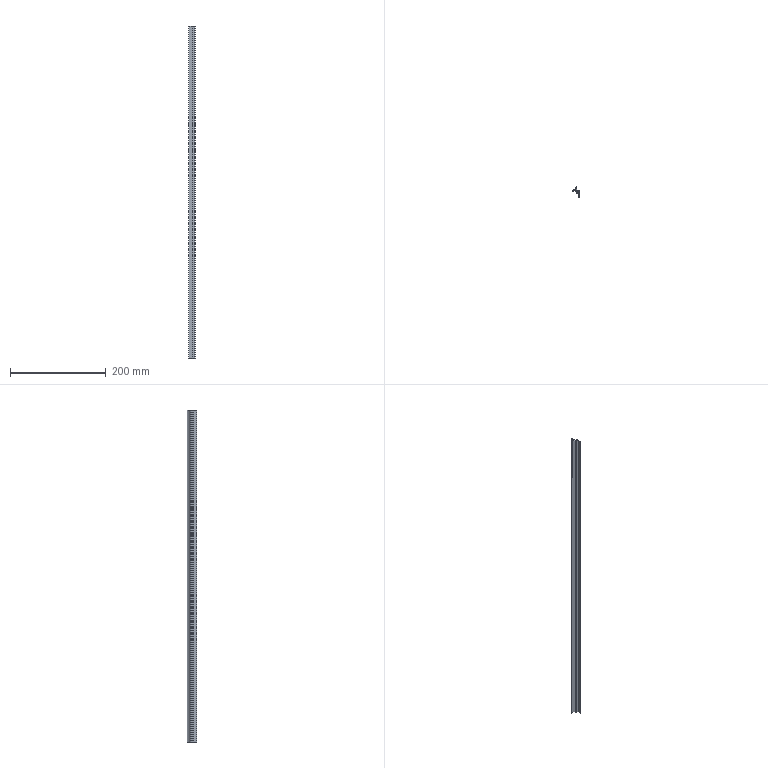Part | SolidWorks | features BaseBody 1, ICE 1, MoveFace 1 | 1 solid | 27 faces | box 14 x 20.3 x 692 mm | volume 35234 mm3 | plane 20 | cylinder 7 | commonest cylinder face diameters 0.387 x2 0.8 x2 0.4 x1 20 x1 22 x1
STEP:
#1=CARTESIAN_POINT('',(-5.304,-0.625,200.));
#2=VERTEX_POINT('',#1);
#3=CARTESIAN_POINT('',(-5.449,-0.8125,200.));
#4=VERTEX_POINT('',#3);
#5=CARTESIAN_POINT('',(-5.255,-0.8125,200.));
#6=DIRECTION('',(0.,0.,1.));
#7=DIRECTION('',(-1.,0.,0.));
#8=AXIS2_PLACEMENT_3D('',#5,#6,#7);
#9=CIRCLE('',#8,0.1937);
#10=EDGE_CURVE('',#2,#4,#9,.T.);
#11=ORIENTED_EDGE('',*,*,#10,.T.);
#12=CARTESIAN_POINT('',(-5.449,-0.8125,-492.));
#13=VERTEX_POINT('',#12);
#14=CARTESIAN_POINT('',(-5.449,-0.8125,230.));
#15=DIRECTION('',(0.,0.,-1.));
#16=VECTOR('',#15,1000.);
#17=LINE('',#14,#16);
#18=EDGE_CURVE('',#4,#13,#17,.T.);
#19=ORIENTED_EDGE('',*,*,#18,.T.);
#20=CARTESIAN_POINT('',(-5.304,-0.625,-492.));
#21=VERTEX_POINT('',#20);
#22=CARTESIAN_POINT('',(-5.255,-0.8125,-492.));
#23=DIRECTION('',(0.,0.,-1.));
#24=DIRECTION('',(1.,0.,0.));
#25=AXIS2_PLACEMENT_3D('',#22,#23,#24);
#26=CIRCLE('',#25,0.1937);
#27=EDGE_CURVE('',#13,#21,#26,.T.);
#28=ORIENTED_EDGE('',*,*,#27,.T.);
#29=CARTESIAN_POINT('',(-5.304,-0.625,230.));
#30=DIRECTION('',(0.,0.,-1.));
#31=VECTOR('',#30,1000.);
#32=LINE('',#29,#31);
#33=EDGE_CURVE('',#2,#21,#32,.T.);
#34=ORIENTED_EDGE('',*,*,#33,.F.);
#35=EDGE_LOOP('',(#11,#19,#28,#34));
#36=FACE_OUTER_BOUND('',#35,.T.);
#37=CARTESIAN_POINT('',(-5.255,-0.8125,230.));
#38=DIRECTION('',(0.,0.,-1.));
#39=DIRECTION('',(-1.,0.,0.));
#40=AXIS2_PLACEMENT_3D('',#37,#38,#39);
#41=CYLINDRICAL_SURFACE('',#40,0.1937);
#42=ADVANCED_FACE('',(#36),#41,.F.);
#43=CARTESIAN_POINT('',(5.,-1.,-492.));
#44=VERTEX_POINT('',#43);
#45=CARTESIAN_POINT('',(5.,-14.3,-492.));
#46=VERTEX_POINT('',#45);
#47=CARTESIAN_POINT('',(5.,29.623,-492.));
#48=DIRECTION('',(0.,-1.,0.));
#49=VECTOR('',#48,1000.);
#50=LINE('',#47,#49);
#51=EDGE_CURVE('',#44,#46,#50,.T.);
#52=ORIENTED_EDGE('',*,*,#51,.F.);
#53=CARTESIAN_POINT('',(5.,-1.,200.));
#54=VERTEX_POINT('',#53);
#55=CARTESIAN_POINT('',(5.,-1.,230.));
#56=DIRECTION('',(0.,0.,-1.));
#57=VECTOR('',#56,1000.);
#58=LINE('',#55,#57);
#59=EDGE_CURVE('',#54,#44,#58,.T.);
#60=ORIENTED_EDGE('',*,*,#59,.F.);
#61=CARTESIAN_POINT('',(5.,-14.3,200.));
#62=VERTEX_POINT('',#61);
#63=CARTESIAN_POINT('',(5.,-14.3,200.));
#64=DIRECTION('',(0.,1.,0.));
#65=VECTOR('',#64,1000.);
#66=LINE('',#63,#65);
#67=EDGE_CURVE('',#62,#54,#66,.T.);
#68=ORIENTED_EDGE('',*,*,#67,.F.);
#69=CARTESIAN_POINT('',(5.,-14.3,230.));
#70=DIRECTION('',(0.,0.,1.));
#71=VECTOR('',#70,1000.);
#72=LINE('',#69,#71);
#73=EDGE_CURVE('',#46,#62,#72,.T.);
#74=ORIENTED_EDGE('',*,*,#73,.F.);
#75=EDGE_LOOP('',(#52,#60,#68,#74));
#76=FACE_OUTER_BOUND('',#75,.T.);
#77=CARTESIAN_POINT('',(5.,-14.3,230.));
#78=DIRECTION('',(-1.,0.,0.));
#79=DIRECTION('',(0.,0.,1.));
#80=AXIS2_PLACEMENT_3D('',#77,#78,#79);
#81=PLANE('',#80);
#82=ADVANCED_FACE('',(#76),#81,.F.);
#83=CARTESIAN_POINT('',(-9.,-2.,-492.));
#84=VERTEX_POINT('',#83);
#85=CARTESIAN_POINT('',(-9.,-2.,200.));
#86=VERTEX_POINT('',#85);
#87=CARTESIAN_POINT('',(-9.,-2.,230.));
#88=DIRECTION('',(0.,0.,1.));
#89=VECTOR('',#88,1000.);
#90=LINE('',#87,#89);
#91=EDGE_CURVE('',#84,#86,#90,.T.);
#92=ORIENTED_EDGE('',*,*,#91,.F.);
#93=CARTESIAN_POINT('',(0.9,-2.,-492.));
#94=VERTEX_POINT('',#93);
#95=CARTESIAN_POINT('',(5.,-2.,-492.));
#96=DIRECTION('',(-1.,0.,0.));
#97=VECTOR('',#96,1000.);
#98=LINE('',#95,#97);
#99=EDGE_CURVE('',#94,#84,#98,.T.);
#100=ORIENTED_EDGE('',*,*,#99,.F.);
#101=CARTESIAN_POINT('',(0.9,-2.,200.));
#102=VERTEX_POINT('',#101);
#103=CARTESIAN_POINT('',(0.9,-2.,230.));
#104=DIRECTION('',(0.,0.,-1.));
#105=VECTOR('',#104,1000.);
#106=LINE('',#103,#105);
#107=EDGE_CURVE('',#102,#94,#106,.T.);
#108=ORIENTED_EDGE('',*,*,#107,.F.);
#109=CARTESIAN_POINT('',(5.,-2.,200.));
#110=DIRECTION('',(1.,0.,0.));
#111=VECTOR('',#110,1000.);
#112=LINE('',#109,#111);
#113=EDGE_CURVE('',#86,#102,#112,.T.);
#114=ORIENTED_EDGE('',*,*,#113,.F.);
#115=EDGE_LOOP('',(#92,#100,#108,#114));
#116=FACE_OUTER_BOUND('',#115,.T.);
#117=CARTESIAN_POINT('',(-9.,-2.,230.));
#118=DIRECTION('',(0.,1.,0.));
#119=DIRECTION('',(0.,0.,1.));
#120=AXIS2_PLACEMENT_3D('',#117,#118,#119);
#121=PLANE('',#120);
#122=ADVANCED_FACE('',(#116),#121,.F.);
#123=CARTESIAN_POINT('',(4.,-6.,200.));
#124=VERTEX_POINT('',#123);
#125=CARTESIAN_POINT('',(4.,-3.,200.));
#126=VERTEX_POINT('',#125);
#127=CARTESIAN_POINT('',(4.,29.623,200.));
#128=DIRECTION('',(0.,1.,0.));
#129=VECTOR('',#128,1000.);
#130=LINE('',#127,#129);
#131=EDGE_CURVE('',#124,#126,#130,.T.);
#132=ORIENTED_EDGE('',*,*,#131,.F.);
#133=CARTESIAN_POINT('',(1.,-6.,200.));
#134=VERTEX_POINT('',#133);
#135=CARTESIAN_POINT('',(5.,-6.,200.));
#136=DIRECTION('',(1.,0.,0.));
#137=VECTOR('',#136,1000.);
#138=LINE('',#135,#137);
#139=EDGE_CURVE('',#134,#124,#138,.T.);
#140=ORIENTED_EDGE('',*,*,#139,.F.);
#141=CARTESIAN_POINT('',(1.,-6.7,200.));
#142=VERTEX_POINT('',#141);
#143=CARTESIAN_POINT('',(1.,-6.,200.));
#144=DIRECTION('',(0.,-1.,0.));
#145=VECTOR('',#144,1000.);
#146=LINE('',#143,#145);
#147=EDGE_CURVE('',#134,#142,#146,.T.);
#148=ORIENTED_EDGE('',*,*,#147,.T.);
#149=CARTESIAN_POINT('',(-1.7,-6.7,200.));
#150=VERTEX_POINT('',#149);
#151=CARTESIAN_POINT('',(5.,-6.7,200.));
#152=DIRECTION('',(1.,0.,0.));
#153=VECTOR('',#152,1000.);
#154=LINE('',#151,#153);
#155=EDGE_CURVE('',#150,#142,#154,.T.);
#156=ORIENTED_EDGE('',*,*,#155,.F.);
#157=CARTESIAN_POINT('',(-1.7,-7.7,200.));
#158=VERTEX_POINT('',#157);
#159=CARTESIAN_POINT('',(-1.7,-6.7,200.));
#160=DIRECTION('',(0.,-1.,0.));
#161=VECTOR('',#160,1000.);
#162=LINE('',#159,#161);
#163=EDGE_CURVE('',#150,#158,#162,.T.);
#164=ORIENTED_EDGE('',*,*,#163,.T.);
#165=CARTESIAN_POINT('',(4.,-7.7,200.));
#166=VERTEX_POINT('',#165);
#167=CARTESIAN_POINT('',(5.,-7.7,200.));
#168=DIRECTION('',(-1.,0.,0.));
#169=VECTOR('',#168,1000.);
#170=LINE('',#167,#169);
#171=EDGE_CURVE('',#166,#158,#170,.T.);
#172=ORIENTED_EDGE('',*,*,#171,.F.);
#173=CARTESIAN_POINT('',(4.,-14.3,200.));
#174=VERTEX_POINT('',#173);
#175=CARTESIAN_POINT('',(4.,29.623,200.));
#176=DIRECTION('',(0.,1.,0.));
#177=VECTOR('',#176,1000.);
#178=LINE('',#175,#177);
#179=EDGE_CURVE('',#174,#166,#178,.T.);
#180=ORIENTED_EDGE('',*,*,#179,.F.);
#181=CARTESIAN_POINT('',(5.,-14.3,200.));
#182=DIRECTION('',(-1.,0.,0.));
#183=VECTOR('',#182,1000.);
#184=LINE('',#181,#183);
#185=EDGE_CURVE('',#62,#174,#184,.T.);
#186=ORIENTED_EDGE('',*,*,#185,.F.);
#187=ORIENTED_EDGE('',*,*,#67,.T.);
#188=CARTESIAN_POINT('',(-5.207,-1.,200.));
#189=VERTEX_POINT('',#188);
#190=CARTESIAN_POINT('',(5.,-1.,200.));
#191=DIRECTION('',(1.,0.,0.));
#192=VECTOR('',#191,1000.);
#193=LINE('',#190,#192);
#194=EDGE_CURVE('',#189,#54,#193,.T.);
#195=ORIENTED_EDGE('',*,*,#194,.F.);
#196=CARTESIAN_POINT('',(-5.255,-0.8125,200.));
#197=DIRECTION('',(0.,0.,1.));
#198=DIRECTION('',(-1.,0.,0.));
#199=AXIS2_PLACEMENT_3D('',#196,#197,#198);
#200=CIRCLE('',#199,0.1937);
#201=EDGE_CURVE('',#4,#189,#200,.T.);
#202=ORIENTED_EDGE('',*,*,#201,.F.);
#203=ORIENTED_EDGE('',*,*,#10,.F.);
#204=CARTESIAN_POINT('',(-1.368,3.063,200.));
#205=VERTEX_POINT('',#204);
#206=CARTESIAN_POINT('',(-10.628,9.,200.));
#207=DIRECTION('',(0.,0.,1.));
#208=DIRECTION('',(-1.,0.,0.));
#209=AXIS2_PLACEMENT_3D('',#206,#207,#208);
#210=CIRCLE('',#209,11.);
#211=EDGE_CURVE('',#2,#205,#210,.T.);
#212=ORIENTED_EDGE('',*,*,#211,.T.);
#213=CARTESIAN_POINT('',(-1.,2.955,200.));
#214=VERTEX_POINT('',#213);
#215=CARTESIAN_POINT('',(-1.2,2.955,200.));
#216=DIRECTION('',(0.,0.,1.));
#217=DIRECTION('',(-1.,0.,0.));
#218=AXIS2_PLACEMENT_3D('',#215,#216,#217);
#219=CIRCLE('',#218,0.2);
#220=EDGE_CURVE('',#214,#205,#219,.T.);
#221=ORIENTED_EDGE('',*,*,#220,.F.);
#222=CARTESIAN_POINT('',(-1.,1.5,200.));
#223=VERTEX_POINT('',#222);
#224=CARTESIAN_POINT('',(-1.,2.955,200.));
#225=DIRECTION('',(0.,1.,0.));
#226=VECTOR('',#225,1000.);
#227=LINE('',#224,#226);
#228=EDGE_CURVE('',#223,#214,#227,.T.);
#229=ORIENTED_EDGE('',*,*,#228,.F.);
#230=CARTESIAN_POINT('',(0.,1.5,200.));
#231=VERTEX_POINT('',#230);
#232=CARTESIAN_POINT('',(-1.,1.5,200.));
#233=DIRECTION('',(-1.,0.,0.));
#234=VECTOR('',#233,1000.);
#235=LINE('',#232,#234);
#236=EDGE_CURVE('',#231,#223,#235,.T.);
#237=ORIENTED_EDGE('',*,*,#236,.F.);
#238=CARTESIAN_POINT('',(0.,6.,200.));
#239=VERTEX_POINT('',#238);
#240=CARTESIAN_POINT('',(0.,1.5,200.));
#241=DIRECTION('',(0.,-1.,0.));
#242=VECTOR('',#241,1000.);
#243=LINE('',#240,#242);
#244=EDGE_CURVE('',#239,#231,#243,.T.);
#245=ORIENTED_EDGE('',*,*,#244,.F.);
#246=CARTESIAN_POINT('',(-0.8,6.,200.));
#247=VERTEX_POINT('',#246);
#248=CARTESIAN_POINT('',(0.,6.,200.));
#249=DIRECTION('',(1.,0.,0.));
#250=VECTOR('',#249,1000.);
#251=LINE('',#248,#250);
#252=EDGE_CURVE('',#247,#239,#251,.T.);
#253=ORIENTED_EDGE('',*,*,#252,.F.);
#254=CARTESIAN_POINT('',(-1.178,5.731,200.));
#255=VERTEX_POINT('',#254);
#256=CARTESIAN_POINT('',(-0.8,5.6,200.));
#257=DIRECTION('',(0.,0.,1.));
#258=DIRECTION('',(-1.,0.,0.));
#259=AXIS2_PLACEMENT_3D('',#256,#257,#258);
#260=CIRCLE('',#259,0.4);
#261=EDGE_CURVE('',#247,#255,#260,.T.);
#262=ORIENTED_EDGE('',*,*,#261,.T.);
#263=CARTESIAN_POINT('',(-8.678,-0.8077,200.));
#264=VERTEX_POINT('',#263);
#265=CARTESIAN_POINT('',(-10.628,9.,200.));
#266=DIRECTION('',(0.,0.,1.));
#267=DIRECTION('',(-1.,0.,0.));
#268=AXIS2_PLACEMENT_3D('',#265,#266,#267);
#269=CIRCLE('',#268,10.);
#270=EDGE_CURVE('',#264,#255,#269,.T.);
#271=ORIENTED_EDGE('',*,*,#270,.F.);
#272=CARTESIAN_POINT('',(-9.,-1.2,200.));
#273=VERTEX_POINT('',#272);
#274=CARTESIAN_POINT('',(-8.6,-1.2,200.));
#275=DIRECTION('',(0.,0.,1.));
#276=DIRECTION('',(-1.,0.,0.));
#277=AXIS2_PLACEMENT_3D('',#274,#275,#276);
#278=CIRCLE('',#277,0.4);
#279=EDGE_CURVE('',#264,#273,#278,.T.);
#280=ORIENTED_EDGE('',*,*,#279,.T.);
#281=CARTESIAN_POINT('',(-9.,8.,200.));
#282=DIRECTION('',(0.,-1.,0.));
#283=VECTOR('',#282,1000.);
#284=LINE('',#281,#283);
#285=EDGE_CURVE('',#273,#86,#284,.T.);
#286=ORIENTED_EDGE('',*,*,#285,.T.);
#287=ORIENTED_EDGE('',*,*,#113,.T.);
#288=CARTESIAN_POINT('',(0.9,-3.,200.));
#289=VERTEX_POINT('',#288);
#290=CARTESIAN_POINT('',(0.9,29.623,200.));
#291=DIRECTION('',(0.,1.,0.));
#292=VECTOR('',#291,1000.);
#293=LINE('',#290,#292);
#294=EDGE_CURVE('',#289,#102,#293,.T.);
#295=ORIENTED_EDGE('',*,*,#294,.F.);
#296=CARTESIAN_POINT('',(5.,-3.,200.));
#297=DIRECTION('',(-1.,0.,0.));
#298=VECTOR('',#297,1000.);
#299=LINE('',#296,#298);
#300=EDGE_CURVE('',#126,#289,#299,.T.);
#301=ORIENTED_EDGE('',*,*,#300,.F.);
#302=EDGE_LOOP('',(#132,#140,#148,#156,#164,#172,#180,#186,#187,#195,#202,#203,#212,#221,#229,#237,#245,#253,#262,#271,#280,#286,#287,#295,#301));
#303=FACE_OUTER_BOUND('',#302,.T.);
#304=CARTESIAN_POINT('',(5.,29.623,200.));
#305=DIRECTION('',(0.,0.,-1.));
#306=DIRECTION('',(-1.,0.,0.));
#307=AXIS2_PLACEMENT_3D('',#304,#305,#306);
#308=PLANE('',#307);
#309=ADVANCED_FACE('',(#303),#308,.F.);
#310=ORIENTED_EDGE('',*,*,#185,.T.);
#311=CARTESIAN_POINT('',(4.,-14.3,-492.));
#312=VERTEX_POINT('',#311);
#313=CARTESIAN_POINT('',(4.,-14.3,230.));
#314=DIRECTION('',(0.,0.,1.));
#315=VECTOR('',#314,1000.);
#316=LINE('',#313,#315);
#317=EDGE_CURVE('',#312,#174,#316,.T.);
#318=ORIENTED_EDGE('',*,*,#317,.F.);
#319=CARTESIAN_POINT('',(5.,-14.3,-492.));
#320=DIRECTION('',(-1.,0.,0.));
#321=VECTOR('',#320,1000.);
#322=LINE('',#319,#321);
#323=EDGE_CURVE('',#46,#312,#322,.T.);
#324=ORIENTED_EDGE('',*,*,#323,.F.);
#325=ORIENTED_EDGE('',*,*,#73,.T.);
#326=EDGE_LOOP('',(#310,#318,#324,#325));
#327=FACE_OUTER_BOUND('',#326,.T.);
#328=CARTESIAN_POINT('',(4.,-14.3,230.));
#329=DIRECTION('',(0.,1.,0.));
#330=DIRECTION('',(0.,0.,1.));
#331=AXIS2_PLACEMENT_3D('',#328,#329,#330);
#332=PLANE('',#331);
#333=ADVANCED_FACE('',(#327),#332,.F.);
#334=ORIENTED_EDGE('',*,*,#51,.T.);
#335=ORIENTED_EDGE('',*,*,#323,.T.);
#336=CARTESIAN_POINT('',(4.,-7.7,-492.));
#337=VERTEX_POINT('',#336);
#338=CARTESIAN_POINT('',(4.,-7.7,-492.));
#339=DIRECTION('',(0.,-1.,0.));
#340=VECTOR('',#339,1000.);
#341=LINE('',#338,#340);
#342=EDGE_CURVE('',#337,#312,#341,.T.);
#343=ORIENTED_EDGE('',*,*,#342,.F.);
#344=CARTESIAN_POINT('',(-1.7,-7.7,-492.));
#345=VERTEX_POINT('',#344);
#346=CARTESIAN_POINT('',(-1.7,-7.7,-492.));
#347=DIRECTION('',(1.,0.,0.));
#348=VECTOR('',#347,1000.);
#349=LINE('',#346,#348);
#350=EDGE_CURVE('',#345,#337,#349,.T.);
#351=ORIENTED_EDGE('',*,*,#350,.F.);
#352=CARTESIAN_POINT('',(-1.7,-6.7,-492.));
#353=VERTEX_POINT('',#352);
#354=CARTESIAN_POINT('',(-1.7,29.623,-492.));
#355=DIRECTION('',(0.,1.,0.));
#356=VECTOR('',#355,1000.);
#357=LINE('',#354,#356);
#358=EDGE_CURVE('',#345,#353,#357,.T.);
#359=ORIENTED_EDGE('',*,*,#358,.T.);
#360=CARTESIAN_POINT('',(1.,-6.7,-492.));
#361=VERTEX_POINT('',#360);
#362=CARTESIAN_POINT('',(1.,-6.7,-492.));
#363=DIRECTION('',(-1.,0.,0.));
#364=VECTOR('',#363,1000.);
#365=LINE('',#362,#364);
#366=EDGE_CURVE('',#361,#353,#365,.T.);
#367=ORIENTED_EDGE('',*,*,#366,.F.);
#368=CARTESIAN_POINT('',(1.,-6.,-492.));
#369=VERTEX_POINT('',#368);
#370=CARTESIAN_POINT('',(1.,29.623,-492.));
#371=DIRECTION('',(0.,1.,0.));
#372=VECTOR('',#371,1000.);
#373=LINE('',#370,#372);
#374=EDGE_CURVE('',#361,#369,#373,.T.);
#375=ORIENTED_EDGE('',*,*,#374,.T.);
#376=CARTESIAN_POINT('',(4.,-6.,-492.));
#377=VERTEX_POINT('',#376);
#378=CARTESIAN_POINT('',(4.,-6.,-492.));
#379=DIRECTION('',(-1.,0.,0.));
#380=VECTOR('',#379,1000.);
#381=LINE('',#378,#380);
#382=EDGE_CURVE('',#377,#369,#381,.T.);
#383=ORIENTED_EDGE('',*,*,#382,.F.);
#384=CARTESIAN_POINT('',(4.,-3.,-492.));
#385=VERTEX_POINT('',#384);
#386=CARTESIAN_POINT('',(4.,-3.,-492.));
#387=DIRECTION('',(0.,-1.,0.));
#388=VECTOR('',#387,1000.);
#389=LINE('',#386,#388);
#390=EDGE_CURVE('',#385,#377,#389,.T.);
#391=ORIENTED_EDGE('',*,*,#390,.F.);
#392=CARTESIAN_POINT('',(0.9,-3.,-492.));
#393=VERTEX_POINT('',#392);
#394=CARTESIAN_POINT('',(0.9,-3.,-492.));
#395=DIRECTION('',(1.,0.,0.));
#396=VECTOR('',#395,1000.);
#397=LINE('',#394,#396);
#398=EDGE_CURVE('',#393,#385,#397,.T.);
#399=ORIENTED_EDGE('',*,*,#398,.F.);
#400=CARTESIAN_POINT('',(0.9,-2.,-492.));
#401=DIRECTION('',(0.,-1.,0.));
#402=VECTOR('',#401,1000.);
#403=LINE('',#400,#402);
#404=EDGE_CURVE('',#94,#393,#403,.T.);
#405=ORIENTED_EDGE('',*,*,#404,.F.);
#406=ORIENTED_EDGE('',*,*,#99,.T.);
#407=CARTESIAN_POINT('',(-9.,-1.2,-492.));
#408=VERTEX_POINT('',#407);
#409=CARTESIAN_POINT('',(-9.,-1.2,-492.));
#410=DIRECTION('',(0.,-1.,0.));
#411=VECTOR('',#410,1000.);
#412=LINE('',#409,#411);
#413=EDGE_CURVE('',#408,#84,#412,.T.);
#414=ORIENTED_EDGE('',*,*,#413,.F.);
#415=CARTESIAN_POINT('',(-8.678,-0.8077,-492.));
#416=VERTEX_POINT('',#415);
#417=CARTESIAN_POINT('',(-8.6,-1.2,-492.));
#418=DIRECTION('',(0.,0.,-1.));
#419=DIRECTION('',(1.,0.,0.));
#420=AXIS2_PLACEMENT_3D('',#417,#418,#419);
#421=CIRCLE('',#420,0.4);
#422=EDGE_CURVE('',#408,#416,#421,.T.);
#423=ORIENTED_EDGE('',*,*,#422,.T.);
#424=CARTESIAN_POINT('',(-1.178,5.731,-492.));
#425=VERTEX_POINT('',#424);
#426=CARTESIAN_POINT('',(-10.628,9.,-492.));
#427=DIRECTION('',(0.,0.,-1.));
#428=DIRECTION('',(1.,0.,0.));
#429=AXIS2_PLACEMENT_3D('',#426,#427,#428);
#430=CIRCLE('',#429,10.);
#431=EDGE_CURVE('',#425,#416,#430,.T.);
#432=ORIENTED_EDGE('',*,*,#431,.F.);
#433=CARTESIAN_POINT('',(-0.8,6.,-492.));
#434=VERTEX_POINT('',#433);
#435=CARTESIAN_POINT('',(-0.8,5.6,-492.));
#436=DIRECTION('',(0.,0.,-1.));
#437=DIRECTION('',(1.,0.,0.));
#438=AXIS2_PLACEMENT_3D('',#435,#436,#437);
#439=CIRCLE('',#438,0.4);
#440=EDGE_CURVE('',#425,#434,#439,.T.);
#441=ORIENTED_EDGE('',*,*,#440,.T.);
#442=CARTESIAN_POINT('',(0.,6.,-492.));
#443=VERTEX_POINT('',#442);
#444=CARTESIAN_POINT('',(0.,6.,-492.));
#445=DIRECTION('',(-1.,0.,0.));
#446=VECTOR('',#445,1000.);
#447=LINE('',#444,#446);
#448=EDGE_CURVE('',#443,#434,#447,.T.);
#449=ORIENTED_EDGE('',*,*,#448,.F.);
#450=CARTESIAN_POINT('',(0.,1.5,-492.));
#451=VERTEX_POINT('',#450);
#452=CARTESIAN_POINT('',(0.,1.5,-492.));
#453=DIRECTION('',(0.,1.,0.));
#454=VECTOR('',#453,1000.);
#455=LINE('',#452,#454);
#456=EDGE_CURVE('',#451,#443,#455,.T.);
#457=ORIENTED_EDGE('',*,*,#456,.F.);
#458=CARTESIAN_POINT('',(-1.,1.5,-492.));
#459=VERTEX_POINT('',#458);
#460=CARTESIAN_POINT('',(-1.,1.5,-492.));
#461=DIRECTION('',(1.,0.,0.));
#462=VECTOR('',#461,1000.);
#463=LINE('',#460,#462);
#464=EDGE_CURVE('',#459,#451,#463,.T.);
#465=ORIENTED_EDGE('',*,*,#464,.F.);
#466=CARTESIAN_POINT('',(-1.,2.955,-492.));
#467=VERTEX_POINT('',#466);
#468=CARTESIAN_POINT('',(-1.,2.955,-492.));
#469=DIRECTION('',(0.,-1.,0.));
#470=VECTOR('',#469,1000.);
#471=LINE('',#468,#470);
#472=EDGE_CURVE('',#467,#459,#471,.T.);
#473=ORIENTED_EDGE('',*,*,#472,.F.);
#474=CARTESIAN_POINT('',(-1.368,3.063,-492.));
#475=VERTEX_POINT('',#474);
#476=CARTESIAN_POINT('',(-1.2,2.955,-492.));
#477=DIRECTION('',(0.,0.,-1.));
#478=DIRECTION('',(1.,0.,0.));
#479=AXIS2_PLACEMENT_3D('',#476,#477,#478);
#480=CIRCLE('',#479,0.2);
#481=EDGE_CURVE('',#475,#467,#480,.T.);
#482=ORIENTED_EDGE('',*,*,#481,.F.);
#483=CARTESIAN_POINT('',(-10.628,9.,-492.));
#484=DIRECTION('',(0.,0.,-1.));
#485=DIRECTION('',(1.,0.,0.));
#486=AXIS2_PLACEMENT_3D('',#483,#484,#485);
#487=CIRCLE('',#486,11.);
#488=EDGE_CURVE('',#475,#21,#487,.T.);
#489=ORIENTED_EDGE('',*,*,#488,.T.);
#490=ORIENTED_EDGE('',*,*,#27,.F.);
#491=CARTESIAN_POINT('',(-5.207,-1.,-492.));
#492=VERTEX_POINT('',#491);
#493=CARTESIAN_POINT('',(-5.255,-0.8125,-492.));
#494=DIRECTION('',(0.,0.,-1.));
#495=DIRECTION('',(1.,0.,0.));
#496=AXIS2_PLACEMENT_3D('',#493,#494,#495);
#497=CIRCLE('',#496,0.1937);
#498=EDGE_CURVE('',#492,#13,#497,.T.);
#499=ORIENTED_EDGE('',*,*,#498,.F.);
#500=CARTESIAN_POINT('',(5.,-1.,-492.));
#501=DIRECTION('',(-1.,0.,0.));
#502=VECTOR('',#501,1000.);
#503=LINE('',#500,#502);
#504=EDGE_CURVE('',#44,#492,#503,.T.);
#505=ORIENTED_EDGE('',*,*,#504,.F.);
#506=EDGE_LOOP('',(#334,#335,#343,#351,#359,#367,#375,#383,#391,#399,#405,#406,#414,#423,#432,#441,#449,#457,#465,#473,#482,#489,#490,#499,#505));
#507=FACE_OUTER_BOUND('',#506,.T.);
#508=CARTESIAN_POINT('',(5.,29.623,-492.));
#509=DIRECTION('',(0.,0.,1.));
#510=DIRECTION('',(1.,0.,0.));
#511=AXIS2_PLACEMENT_3D('',#508,#509,#510);
#512=PLANE('',#511);
#513=ADVANCED_FACE('',(#507),#512,.F.);
#514=ORIENTED_EDGE('',*,*,#59,.T.);
#515=ORIENTED_EDGE('',*,*,#504,.T.);
#516=CARTESIAN_POINT('',(-5.207,-1.,230.));
#517=DIRECTION('',(0.,0.,-1.));
#518=VECTOR('',#517,1000.);
#519=LINE('',#516,#518);
#520=EDGE_CURVE('',#189,#492,#519,.T.);
#521=ORIENTED_EDGE('',*,*,#520,.F.);
#522=ORIENTED_EDGE('',*,*,#194,.T.);
#523=EDGE_LOOP('',(#514,#515,#521,#522));
#524=FACE_OUTER_BOUND('',#523,.T.);
#525=CARTESIAN_POINT('',(5.,-1.,230.));
#526=DIRECTION('',(0.,-1.,0.));
#527=DIRECTION('',(0.,0.,-1.));
#528=AXIS2_PLACEMENT_3D('',#525,#526,#527);
#529=PLANE('',#528);
#530=ADVANCED_FACE('',(#524),#529,.F.);
#531=CARTESIAN_POINT('',(-9.,-1.2,230.));
#532=DIRECTION('',(0.,0.,1.));
#533=VECTOR('',#532,1000.);
#534=LINE('',#531,#533);
#535=EDGE_CURVE('',#408,#273,#534,.T.);
#536=ORIENTED_EDGE('',*,*,#535,.F.);
#537=ORIENTED_EDGE('',*,*,#413,.T.);
#538=ORIENTED_EDGE('',*,*,#91,.T.);
#539=ORIENTED_EDGE('',*,*,#285,.F.);
#540=EDGE_LOOP('',(#536,#537,#538,#539));
#541=FACE_OUTER_BOUND('',#540,.T.);
#542=CARTESIAN_POINT('',(-9.,-1.2,230.));
#543=DIRECTION('',(1.,0.,0.));
#544=DIRECTION('',(0.,0.,-1.));
#545=AXIS2_PLACEMENT_3D('',#542,#543,#544);
#546=PLANE('',#545);
#547=ADVANCED_FACE('',(#541),#546,.F.);
#548=ORIENTED_EDGE('',*,*,#294,.T.);
#549=ORIENTED_EDGE('',*,*,#107,.T.);
#550=ORIENTED_EDGE('',*,*,#404,.T.);
#551=CARTESIAN_POINT('',(0.9,-3.,230.));
#552=DIRECTION('',(0.,0.,-1.));
#553=VECTOR('',#552,1000.);
#554=LINE('',#551,#553);
#555=EDGE_CURVE('',#289,#393,#554,.T.);
#556=ORIENTED_EDGE('',*,*,#555,.F.);
#557=EDGE_LOOP('',(#548,#549,#550,#556));
#558=FACE_OUTER_BOUND('',#557,.T.);
#559=CARTESIAN_POINT('',(0.9,-2.,230.));
#560=DIRECTION('',(1.,0.,0.));
#561=DIRECTION('',(0.,0.,-1.));
#562=AXIS2_PLACEMENT_3D('',#559,#560,#561);
#563=PLANE('',#562);
#564=ADVANCED_FACE('',(#558),#563,.F.);
#565=ORIENTED_EDGE('',*,*,#300,.T.);
#566=ORIENTED_EDGE('',*,*,#555,.T.);
#567=ORIENTED_EDGE('',*,*,#398,.T.);
#568=CARTESIAN_POINT('',(4.,-3.,230.));
#569=DIRECTION('',(0.,0.,-1.));
#570=VECTOR('',#569,1000.);
#571=LINE('',#568,#570);
#572=EDGE_CURVE('',#126,#385,#571,.T.);
#573=ORIENTED_EDGE('',*,*,#572,.F.);
#574=EDGE_LOOP('',(#565,#566,#567,#573));
#575=FACE_OUTER_BOUND('',#574,.T.);
#576=CARTESIAN_POINT('',(0.9,-3.,230.));
#577=DIRECTION('',(0.,1.,0.));
#578=DIRECTION('',(0.,0.,1.));
#579=AXIS2_PLACEMENT_3D('',#576,#577,#578);
#580=PLANE('',#579);
#581=ADVANCED_FACE('',(#575),#580,.F.);
#582=ORIENTED_EDGE('',*,*,#131,.T.);
#583=ORIENTED_EDGE('',*,*,#572,.T.);
#584=ORIENTED_EDGE('',*,*,#390,.T.);
#585=CARTESIAN_POINT('',(4.,-6.,230.));
#586=DIRECTION('',(0.,0.,-1.));
#587=VECTOR('',#586,1000.);
#588=LINE('',#585,#587);
#589=EDGE_CURVE('',#124,#377,#588,.T.);
#590=ORIENTED_EDGE('',*,*,#589,.F.);
#591=EDGE_LOOP('',(#582,#583,#584,#590));
#592=FACE_OUTER_BOUND('',#591,.T.);
#593=CARTESIAN_POINT('',(4.,-3.,230.));
#594=DIRECTION('',(1.,0.,0.));
#595=DIRECTION('',(0.,0.,-1.));
#596=AXIS2_PLACEMENT_3D('',#593,#594,#595);
#597=PLANE('',#596);
#598=ADVANCED_FACE('',(#592),#597,.F.);
#599=ORIENTED_EDGE('',*,*,#139,.T.);
#600=ORIENTED_EDGE('',*,*,#589,.T.);
#601=ORIENTED_EDGE('',*,*,#382,.T.);
#602=CARTESIAN_POINT('',(1.,-6.,230.));
#603=DIRECTION('',(0.,0.,-1.));
#604=VECTOR('',#603,1000.);
#605=LINE('',#602,#604);
#606=EDGE_CURVE('',#134,#369,#605,.T.);
#607=ORIENTED_EDGE('',*,*,#606,.F.);
#608=EDGE_LOOP('',(#599,#600,#601,#607));
#609=FACE_OUTER_BOUND('',#608,.T.);
#610=CARTESIAN_POINT('',(4.,-6.,230.));
#611=DIRECTION('',(0.,-1.,0.));
#612=DIRECTION('',(0.,0.,-1.));
#613=AXIS2_PLACEMENT_3D('',#610,#611,#612);
#614=PLANE('',#613);
#615=ADVANCED_FACE('',(#609),#614,.F.);
#616=ORIENTED_EDGE('',*,*,#155,.T.);
#617=CARTESIAN_POINT('',(1.,-6.7,230.));
#618=DIRECTION('',(0.,0.,1.));
#619=VECTOR('',#618,1000.);
#620=LINE('',#617,#619);
#621=EDGE_CURVE('',#361,#142,#620,.T.);
#622=ORIENTED_EDGE('',*,*,#621,.F.);
#623=ORIENTED_EDGE('',*,*,#366,.T.);
#624=CARTESIAN_POINT('',(-1.7,-6.7,230.));
#625=DIRECTION('',(0.,0.,-1.));
#626=VECTOR('',#625,1000.);
#627=LINE('',#624,#626);
#628=EDGE_CURVE('',#150,#353,#627,.T.);
#629=ORIENTED_EDGE('',*,*,#628,.F.);
#630=EDGE_LOOP('',(#616,#622,#623,#629));
#631=FACE_OUTER_BOUND('',#630,.T.);
#632=CARTESIAN_POINT('',(1.,-6.7,230.));
#633=DIRECTION('',(0.,-1.,0.));
#634=DIRECTION('',(0.,0.,-1.));
#635=AXIS2_PLACEMENT_3D('',#632,#633,#634);
#636=PLANE('',#635);
#637=ADVANCED_FACE('',(#631),#636,.F.);
#638=ORIENTED_EDGE('',*,*,#171,.T.);
#639=CARTESIAN_POINT('',(-1.7,-7.7,230.));
#640=DIRECTION('',(0.,0.,1.));
#641=VECTOR('',#640,1000.);
#642=LINE('',#639,#641);
#643=EDGE_CURVE('',#345,#158,#642,.T.);
#644=ORIENTED_EDGE('',*,*,#643,.F.);
#645=ORIENTED_EDGE('',*,*,#350,.T.);
#646=CARTESIAN_POINT('',(4.,-7.7,230.));
#647=DIRECTION('',(0.,0.,-1.));
#648=VECTOR('',#647,1000.);
#649=LINE('',#646,#648);
#650=EDGE_CURVE('',#166,#337,#649,.T.);
#651=ORIENTED_EDGE('',*,*,#650,.F.);
#652=EDGE_LOOP('',(#638,#644,#645,#651));
#653=FACE_OUTER_BOUND('',#652,.T.);
#654=CARTESIAN_POINT('',(-1.7,-7.7,230.));
#655=DIRECTION('',(0.,1.,0.));
#656=DIRECTION('',(0.,0.,1.));
#657=AXIS2_PLACEMENT_3D('',#654,#655,#656);
#658=PLANE('',#657);
#659=ADVANCED_FACE('',(#653),#658,.F.);
#660=ORIENTED_EDGE('',*,*,#179,.T.);
#661=ORIENTED_EDGE('',*,*,#650,.T.);
#662=ORIENTED_EDGE('',*,*,#342,.T.);
#663=ORIENTED_EDGE('',*,*,#317,.T.);
#664=EDGE_LOOP('',(#660,#661,#662,#663));
#665=FACE_OUTER_BOUND('',#664,.T.);
#666=CARTESIAN_POINT('',(4.,-7.7,230.));
#667=DIRECTION('',(1.,0.,0.));
#668=DIRECTION('',(0.,0.,-1.));
#669=AXIS2_PLACEMENT_3D('',#666,#667,#668);
#670=PLANE('',#669);
#671=ADVANCED_FACE('',(#665),#670,.F.);
#672=ORIENTED_EDGE('',*,*,#18,.F.);
#673=ORIENTED_EDGE('',*,*,#201,.T.);
#674=ORIENTED_EDGE('',*,*,#520,.T.);
#675=ORIENTED_EDGE('',*,*,#498,.T.);
#676=EDGE_LOOP('',(#672,#673,#674,#675));
#677=FACE_OUTER_BOUND('',#676,.T.);
#678=CARTESIAN_POINT('',(-5.255,-0.8125,230.));
#679=DIRECTION('',(0.,0.,-1.));
#680=DIRECTION('',(-1.,0.,0.));
#681=AXIS2_PLACEMENT_3D('',#678,#679,#680);
#682=CYLINDRICAL_SURFACE('',#681,0.1937);
#683=ADVANCED_FACE('',(#677),#682,.F.);
#684=CARTESIAN_POINT('',(-1.,2.955,230.));
#685=DIRECTION('',(0.,0.,1.));
#686=VECTOR('',#685,1000.);
#687=LINE('',#684,#686);
#688=EDGE_CURVE('',#467,#214,#687,.T.);
#689=ORIENTED_EDGE('',*,*,#688,.F.);
#690=ORIENTED_EDGE('',*,*,#472,.T.);
#691=CARTESIAN_POINT('',(-1.,1.5,230.));
#692=DIRECTION('',(0.,0.,-1.));
#693=VECTOR('',#692,1000.);
#694=LINE('',#691,#693);
#695=EDGE_CURVE('',#223,#459,#694,.T.);
#696=ORIENTED_EDGE('',*,*,#695,.F.);
#697=ORIENTED_EDGE('',*,*,#228,.T.);
#698=EDGE_LOOP('',(#689,#690,#696,#697));
#699=FACE_OUTER_BOUND('',#698,.T.);
#700=CARTESIAN_POINT('',(-1.,2.955,230.));
#701=DIRECTION('',(1.,0.,0.));
#702=DIRECTION('',(0.,0.,-1.));
#703=AXIS2_PLACEMENT_3D('',#700,#701,#702);
#704=PLANE('',#703);
#705=ADVANCED_FACE('',(#699),#704,.F.);
#706=ORIENTED_EDGE('',*,*,#488,.F.);
#707=CARTESIAN_POINT('',(-1.368,3.063,230.));
#708=DIRECTION('',(0.,0.,1.));
#709=VECTOR('',#708,1000.);
#710=LINE('',#707,#709);
#711=EDGE_CURVE('',#475,#205,#710,.T.);
#712=ORIENTED_EDGE('',*,*,#711,.T.);
#713=ORIENTED_EDGE('',*,*,#211,.F.);
#714=ORIENTED_EDGE('',*,*,#33,.T.);
#715=EDGE_LOOP('',(#706,#712,#713,#714));
#716=FACE_OUTER_BOUND('',#715,.T.);
#717=CARTESIAN_POINT('',(-10.628,9.,230.));
#718=DIRECTION('',(0.,0.,-1.));
#719=DIRECTION('',(-1.,0.,0.));
#720=AXIS2_PLACEMENT_3D('',#717,#718,#719);
#721=CYLINDRICAL_SURFACE('',#720,11.);
#722=ADVANCED_FACE('',(#716),#721,.T.);
#723=CARTESIAN_POINT('',(-1.178,5.731,230.));
#724=DIRECTION('',(0.,0.,1.));
#725=VECTOR('',#724,1000.);
#726=LINE('',#723,#725);
#727=EDGE_CURVE('',#425,#255,#726,.T.);
#728=ORIENTED_EDGE('',*,*,#727,.F.);
#729=ORIENTED_EDGE('',*,*,#431,.T.);
#730=CARTESIAN_POINT('',(-8.678,-0.8077,230.));
#731=DIRECTION('',(0.,0.,-1.));
#732=VECTOR('',#731,1000.);
#733=LINE('',#730,#732);
#734=EDGE_CURVE('',#264,#416,#733,.T.);
#735=ORIENTED_EDGE('',*,*,#734,.F.);
#736=ORIENTED_EDGE('',*,*,#270,.T.);
#737=EDGE_LOOP('',(#728,#729,#735,#736));
#738=FACE_OUTER_BOUND('',#737,.T.);
#739=CARTESIAN_POINT('',(-10.628,9.,230.));
#740=DIRECTION('',(0.,0.,-1.));
#741=DIRECTION('',(-1.,0.,0.));
#742=AXIS2_PLACEMENT_3D('',#739,#740,#741);
#743=CYLINDRICAL_SURFACE('',#742,10.);
#744=ADVANCED_FACE('',(#738),#743,.F.);
#745=CARTESIAN_POINT('',(0.,1.5,230.));
#746=DIRECTION('',(0.,0.,1.));
#747=VECTOR('',#746,1000.);
#748=LINE('',#745,#747);
#749=EDGE_CURVE('',#451,#231,#748,.T.);
#750=ORIENTED_EDGE('',*,*,#749,.F.);
#751=ORIENTED_EDGE('',*,*,#456,.T.);
#752=CARTESIAN_POINT('',(0.,6.,230.));
#753=DIRECTION('',(0.,0.,-1.));
#754=VECTOR('',#753,1000.);
#755=LINE('',#752,#754);
#756=EDGE_CURVE('',#239,#443,#755,.T.);
#757=ORIENTED_EDGE('',*,*,#756,.F.);
#758=ORIENTED_EDGE('',*,*,#244,.T.);
#759=EDGE_LOOP('',(#750,#751,#757,#758));
#760=FACE_OUTER_BOUND('',#759,.T.);
#761=CARTESIAN_POINT('',(0.,1.5,230.));
#762=DIRECTION('',(-1.,0.,0.));
#763=DIRECTION('',(0.,0.,1.));
#764=AXIS2_PLACEMENT_3D('',#761,#762,#763);
#765=PLANE('',#764);
#766=ADVANCED_FACE('',(#760),#765,.F.);
#767=ORIENTED_EDGE('',*,*,#422,.F.);
#768=ORIENTED_EDGE('',*,*,#535,.T.);
#769=ORIENTED_EDGE('',*,*,#279,.F.);
#770=ORIENTED_EDGE('',*,*,#734,.T.);
#771=EDGE_LOOP('',(#767,#768,#769,#770));
#772=FACE_OUTER_BOUND('',#771,.T.);
#773=CARTESIAN_POINT('',(-8.6,-1.2,230.));
#774=DIRECTION('',(0.,0.,-1.));
#775=DIRECTION('',(-1.,0.,0.));
#776=AXIS2_PLACEMENT_3D('',#773,#774,#775);
#777=CYLINDRICAL_SURFACE('',#776,0.4);
#778=ADVANCED_FACE('',(#772),#777,.T.);
#779=ORIENTED_EDGE('',*,*,#147,.F.);
#780=ORIENTED_EDGE('',*,*,#606,.T.);
#781=ORIENTED_EDGE('',*,*,#374,.F.);
#782=ORIENTED_EDGE('',*,*,#621,.T.);
#783=EDGE_LOOP('',(#779,#780,#781,#782));
#784=FACE_OUTER_BOUND('',#783,.T.);
#785=CARTESIAN_POINT('',(1.,-6.,230.));
#786=DIRECTION('',(1.,0.,0.));
#787=DIRECTION('',(0.,0.,-1.));
#788=AXIS2_PLACEMENT_3D('',#785,#786,#787);
#789=PLANE('',#788);
#790=ADVANCED_FACE('',(#784),#789,.F.);
#791=ORIENTED_EDGE('',*,*,#163,.F.);
#792=ORIENTED_EDGE('',*,*,#628,.T.);
#793=ORIENTED_EDGE('',*,*,#358,.F.);
#794=ORIENTED_EDGE('',*,*,#643,.T.);
#795=EDGE_LOOP('',(#791,#792,#793,#794));
#796=FACE_OUTER_BOUND('',#795,.T.);
#797=CARTESIAN_POINT('',(-1.7,-6.7,230.));
#798=DIRECTION('',(1.,0.,0.));
#799=DIRECTION('',(0.,0.,-1.));
#800=AXIS2_PLACEMENT_3D('',#797,#798,#799);
#801=PLANE('',#800);
#802=ADVANCED_FACE('',(#796),#801,.F.);
#803=ORIENTED_EDGE('',*,*,#711,.F.);
#804=ORIENTED_EDGE('',*,*,#481,.T.);
#805=ORIENTED_EDGE('',*,*,#688,.T.);
#806=ORIENTED_EDGE('',*,*,#220,.T.);
#807=EDGE_LOOP('',(#803,#804,#805,#806));
#808=FACE_OUTER_BOUND('',#807,.T.);
#809=CARTESIAN_POINT('',(-1.2,2.955,230.));
#810=DIRECTION('',(0.,0.,-1.));
#811=DIRECTION('',(-1.,0.,0.));
#812=AXIS2_PLACEMENT_3D('',#809,#810,#811);
#813=CYLINDRICAL_SURFACE('',#812,0.2);
#814=ADVANCED_FACE('',(#808),#813,.F.);
#815=ORIENTED_EDGE('',*,*,#695,.T.);
#816=ORIENTED_EDGE('',*,*,#464,.T.);
#817=ORIENTED_EDGE('',*,*,#749,.T.);
#818=ORIENTED_EDGE('',*,*,#236,.T.);
#819=EDGE_LOOP('',(#815,#816,#817,#818));
#820=FACE_OUTER_BOUND('',#819,.T.);
#821=CARTESIAN_POINT('',(-1.,1.5,230.));
#822=DIRECTION('',(0.,1.,0.));
#823=DIRECTION('',(0.,0.,1.));
#824=AXIS2_PLACEMENT_3D('',#821,#822,#823);
#825=PLANE('',#824);
#826=ADVANCED_FACE('',(#820),#825,.F.);
#827=ORIENTED_EDGE('',*,*,#440,.F.);
#828=ORIENTED_EDGE('',*,*,#727,.T.);
#829=ORIENTED_EDGE('',*,*,#261,.F.);
#830=CARTESIAN_POINT('',(-0.8,6.,230.));
#831=DIRECTION('',(0.,0.,-1.));
#832=VECTOR('',#831,1000.);
#833=LINE('',#830,#832);
#834=EDGE_CURVE('',#247,#434,#833,.T.);
#835=ORIENTED_EDGE('',*,*,#834,.T.);
#836=EDGE_LOOP('',(#827,#828,#829,#835));
#837=FACE_OUTER_BOUND('',#836,.T.);
#838=CARTESIAN_POINT('',(-0.8,5.6,230.));
#839=DIRECTION('',(0.,0.,-1.));
#840=DIRECTION('',(-1.,0.,0.));
#841=AXIS2_PLACEMENT_3D('',#838,#839,#840);
#842=CYLINDRICAL_SURFACE('',#841,0.4);
#843=ADVANCED_FACE('',(#837),#842,.T.);
#844=ORIENTED_EDGE('',*,*,#756,.T.);
#845=ORIENTED_EDGE('',*,*,#448,.T.);
#846=ORIENTED_EDGE('',*,*,#834,.F.);
#847=ORIENTED_EDGE('',*,*,#252,.T.);
#848=EDGE_LOOP('',(#844,#845,#846,#847));
#849=FACE_OUTER_BOUND('',#848,.T.);
#850=CARTESIAN_POINT('',(0.,6.,230.));
#851=DIRECTION('',(0.,-1.,0.));
#852=DIRECTION('',(0.,0.,-1.));
#853=AXIS2_PLACEMENT_3D('',#850,#851,#852);
#854=PLANE('',#853);
#855=ADVANCED_FACE('',(#849),#854,.F.);
#856=CLOSED_SHELL('',(#42,#82,#122,#309,#333,#513,#530,#547,#564,#581,#598,#615,#637,#659,#671,#683,#705,#722,#744,#766,#778,#790,#802,#814,#826,#843,#855));
#857=MANIFOLD_SOLID_BREP('',#856);
#858=CARTESIAN_POINT('',(0.,0.,0.));
#859=DIRECTION('',(0.,0.,1.));
#860=DIRECTION('',(1.,0.,0.));
#861=AXIS2_PLACEMENT_3D('',#858,#859,#860);
#862=(LENGTH_UNIT()NAMED_UNIT(*)SI_UNIT(.MILLI.,.METRE.));
#863=UNCERTAINTY_MEASURE_WITH_UNIT(LENGTH_MEASURE(0.00001),#862,'','');
#864=(NAMED_UNIT(*)PLANE_ANGLE_UNIT()SI_UNIT($,.RADIAN.));
#865=(NAMED_UNIT(*)SI_UNIT($,.STERADIAN.)SOLID_ANGLE_UNIT());
#866=(GEOMETRIC_REPRESENTATION_CONTEXT(3)GLOBAL_UNCERTAINTY_ASSIGNED_CONTEXT((#863))GLOBAL_UNIT_ASSIGNED_CONTEXT((#862,#864,#865))REPRESENTATION_CONTEXT('',''));
#867=ADVANCED_BREP_SHAPE_REPRESENTATION('',(#857,#861),#866);